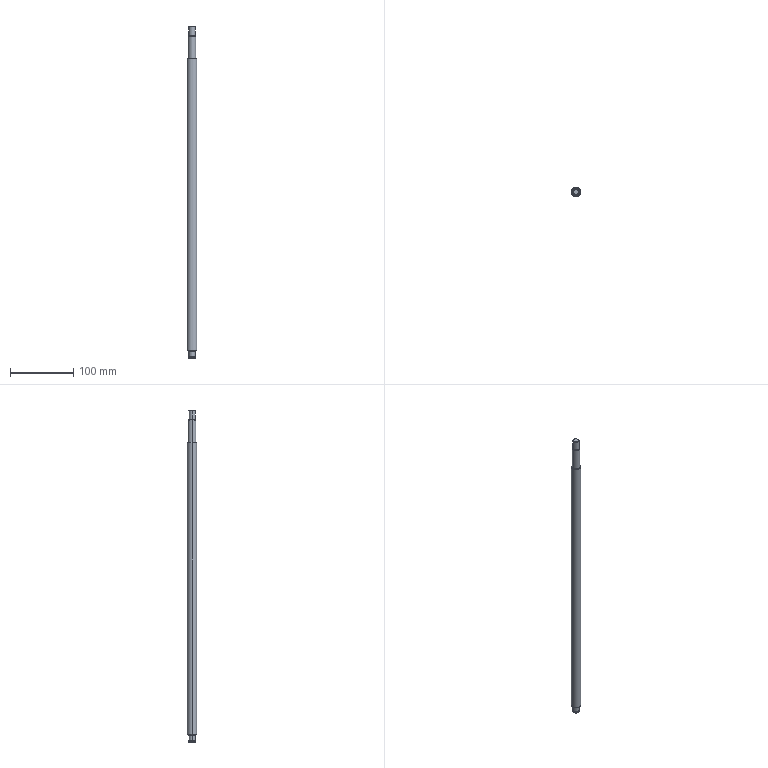Part | STEP file | 1 solid | 28 faces | box 15 x 15 x 523 mm | volume 87491 mm3 | cylinder 12 | cone 10 | plane 6 | commonest cylinder face diameters 10 x6 9.6 x2 12 x2 15 x2